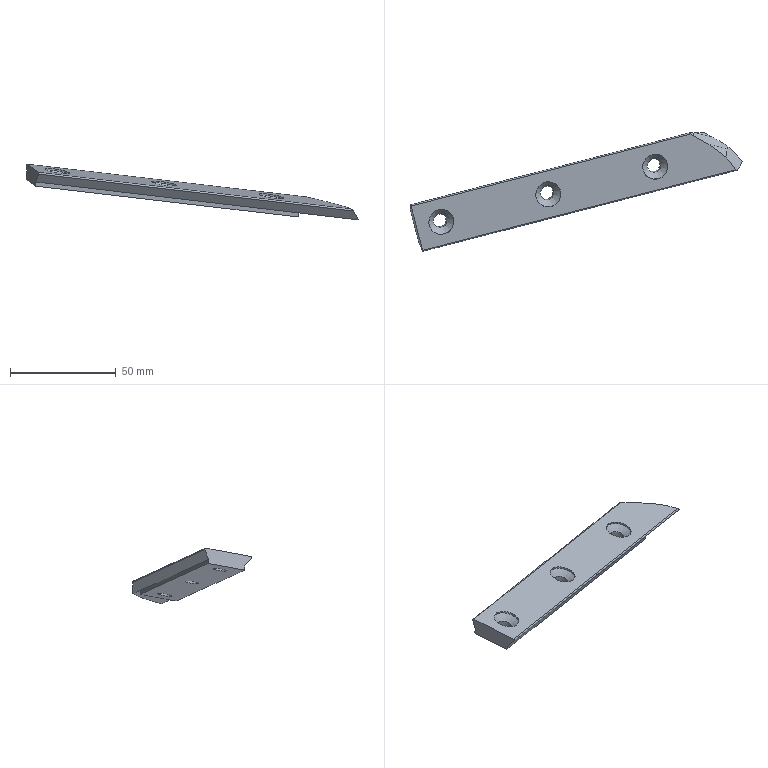Part | STEP file | 车灯-后视镜_id630_x_t | 1 solid | 25 faces | box 156.791 x 56.039 x 26.254 mm | volume 19026 mm3 | plane 9 | cylinder 6 | spline 5 | cone 3 | other 2 | commonest cylinder face diameters 6.5 x3 12 x3